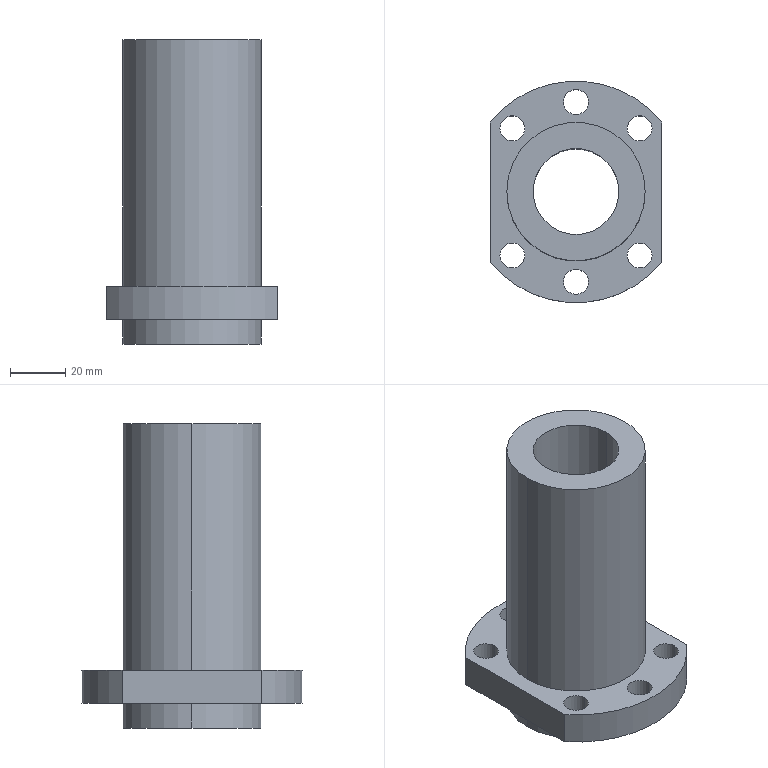Part | STEP file | ball screw nut-SFA3232-2.8 | 1 solid | 26 faces | box 62 x 80 x 110 mm | volume 157675 mm3 | cylinder 20 | plane 6 | commonest cylinder face diameters 9 x12 50 x4 31 x2 80 x2